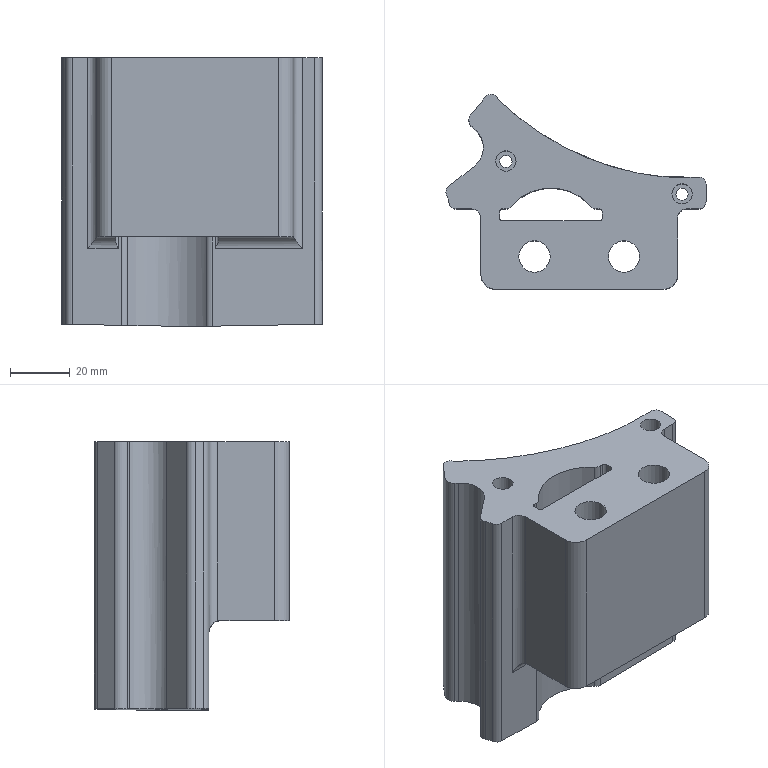Part | STEP file | gslz 2016.10.28-10_id3082_x_t | 1 solid | 54 faces | box 87.187 x 65.37 x 90 mm | volume 204585 mm3 | cylinder 30 | plane 22 | other 2 | commonest cylinder face diameters 5 x8 2 x4 6 x3 4.1 x2 6.8 x2 8 x2